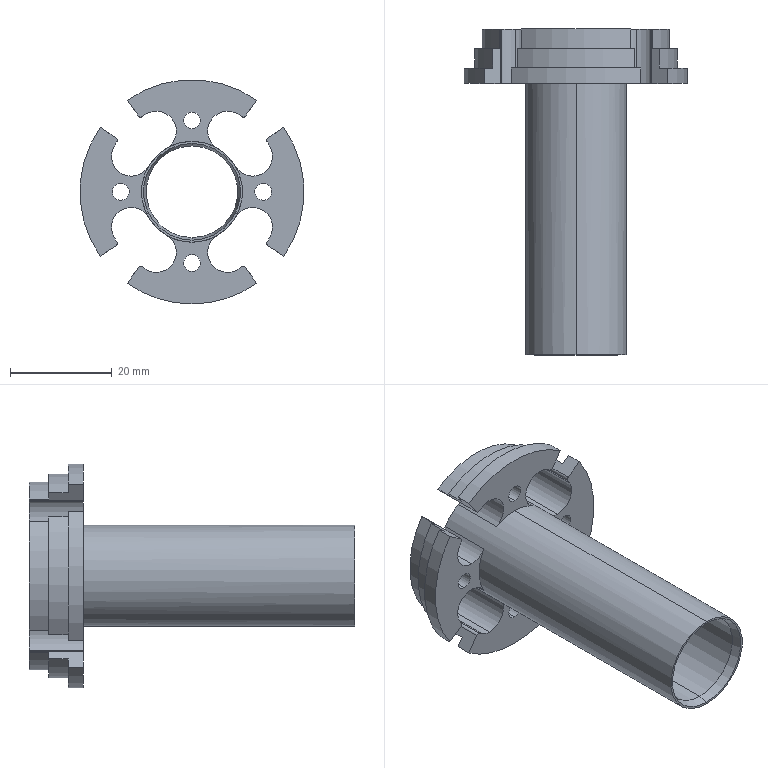Part | SolidWorks | features ICE 3, Chamfer 1, Extrusion 1, Fillet 1, HoleWzd 1 | 1 solid | 81 faces | box 44 x 63.961 x 44 mm | volume 8169 mm3 | cylinder 57 | plane 22 | cone 2 | commonest cylinder face diameters 7.8 x12 1 x10 3.3 x8 35.4 x8 36.9 x5 40 x5